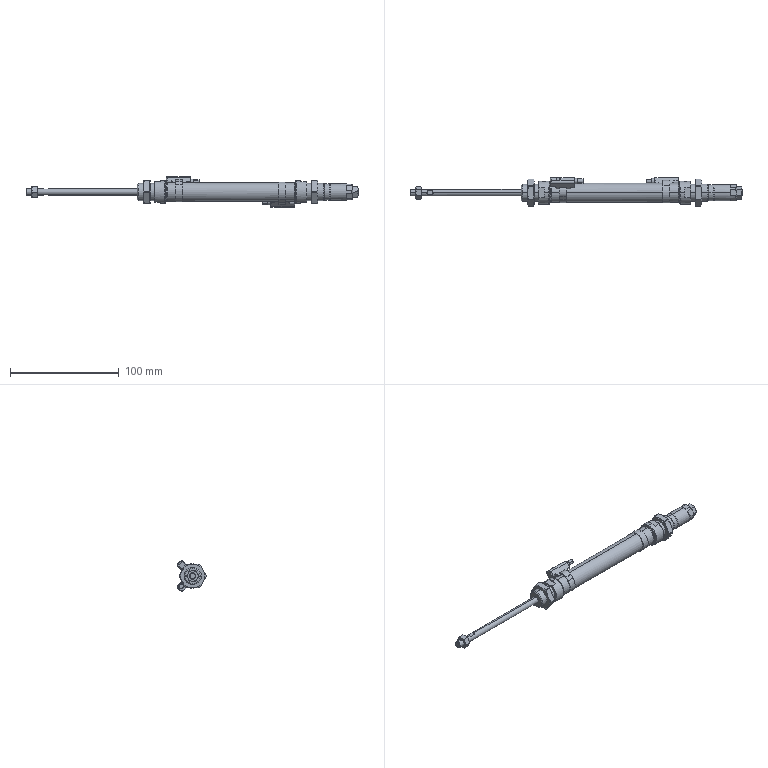Part | SolidWorks | features BaseBody 9, MoveFace 3 | 9 solids | 376 faces | box 305 x 26.327 x 27.654 mm | volume 41177 mm3 | plane 160 | cylinder 108 | cone 84 | spline 24 | commonest cylinder face diameters 3.4 x12 25 x12 2 x8 6 x8 12.4 x8 4.917 x6